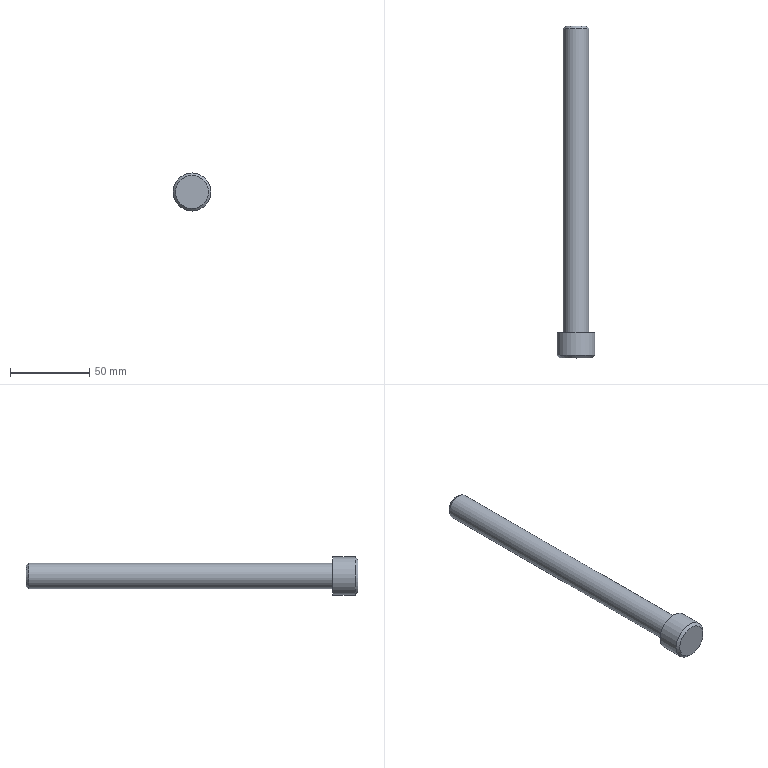Part | STEP file | SCREW-1_id382_x_t | 1 solid | 7 faces | box 24 x 209.351 x 24 mm | volume 45976 mm3 | plane 3 | cone 2 | cylinder 2 | commonest cylinder face diameters 16 x1 24 x1
STEP:
#1=CARTESIAN_POINT('',(165.,-290.,10.4));
#2=VERTEX_POINT('',#1);
#3=CARTESIAN_POINT('',(165.,-290.,0.));
#4=DIRECTION('',(0.,1.,0.));
#5=DIRECTION('',(0.,0.,1.));
#6=AXIS2_PLACEMENT_3D('',#3,#4,#5);
#7=CIRCLE('',#6,10.4);
#8=EDGE_CURVE('',#2,#2,#7,.T.);
#9=ORIENTED_EDGE('',*,*,#8,.F.);
#10=EDGE_LOOP('',(#9));
#11=FACE_OUTER_BOUND('',#10,.T.);
#12=CARTESIAN_POINT('',(165.,-290.,0.));
#13=DIRECTION('',(0.,1.,0.));
#14=DIRECTION('',(0.,0.,1.));
#15=AXIS2_PLACEMENT_3D('',#12,#13,#14);
#16=PLANE('',#15);
#17=ADVANCED_FACE('',(#11),#16,.F.);
#18=CARTESIAN_POINT('',(165.,-288.4,12.));
#19=VERTEX_POINT('',#18);
#20=CARTESIAN_POINT('',(165.,-288.4,0.));
#21=DIRECTION('',(0.,1.,0.));
#22=DIRECTION('',(0.,0.,1.));
#23=AXIS2_PLACEMENT_3D('',#20,#21,#22);
#24=CIRCLE('',#23,12.);
#25=EDGE_CURVE('',#19,#19,#24,.T.);
#26=ORIENTED_EDGE('',*,*,#25,.F.);
#27=EDGE_LOOP('',(#26));
#28=FACE_BOUND('',#27,.T.);
#29=ORIENTED_EDGE('',*,*,#8,.T.);
#30=EDGE_LOOP('',(#29));
#31=FACE_BOUND('',#30,.T.);
#32=CARTESIAN_POINT('',(165.,-288.4,0.));
#33=DIRECTION('',(0.,1.,0.));
#34=DIRECTION('',(0.,0.,1.));
#35=AXIS2_PLACEMENT_3D('',#32,#33,#34);
#36=CONICAL_SURFACE('',#35,12.,45.);
#37=ADVANCED_FACE('',(#28,#31),#36,.T.);
#38=CARTESIAN_POINT('',(165.,-274.,12.));
#39=VERTEX_POINT('',#38);
#40=CARTESIAN_POINT('',(165.,-274.,0.));
#41=DIRECTION('',(0.,1.,0.));
#42=DIRECTION('',(0.,0.,1.));
#43=AXIS2_PLACEMENT_3D('',#40,#41,#42);
#44=CIRCLE('',#43,12.);
#45=EDGE_CURVE('',#39,#39,#44,.T.);
#46=ORIENTED_EDGE('',*,*,#45,.F.);
#47=EDGE_LOOP('',(#46));
#48=FACE_BOUND('',#47,.T.);
#49=ORIENTED_EDGE('',*,*,#25,.T.);
#50=EDGE_LOOP('',(#49));
#51=FACE_BOUND('',#50,.T.);
#52=CARTESIAN_POINT('',(165.,-70.182,0.));
#53=DIRECTION('',(0.,1.,0.));
#54=DIRECTION('',(0.,0.,1.));
#55=AXIS2_PLACEMENT_3D('',#52,#53,#54);
#56=CYLINDRICAL_SURFACE('',#55,12.);
#57=ADVANCED_FACE('',(#48,#51),#56,.T.);
#58=CARTESIAN_POINT('',(165.,-80.649,-6.8));
#59=VERTEX_POINT('',#58);
#60=CARTESIAN_POINT('',(165.,-80.649,0.));
#61=DIRECTION('',(0.,-1.,0.));
#62=DIRECTION('',(0.,0.,-1.));
#63=AXIS2_PLACEMENT_3D('',#60,#61,#62);
#64=CIRCLE('',#63,6.8);
#65=EDGE_CURVE('',#59,#59,#64,.T.);
#66=ORIENTED_EDGE('',*,*,#65,.F.);
#67=EDGE_LOOP('',(#66));
#68=FACE_OUTER_BOUND('',#67,.T.);
#69=CARTESIAN_POINT('',(165.,-80.649,0.));
#70=DIRECTION('',(0.,1.,0.));
#71=DIRECTION('',(0.,0.,1.));
#72=AXIS2_PLACEMENT_3D('',#69,#70,#71);
#73=PLANE('',#72);
#74=ADVANCED_FACE('',(#68),#73,.T.);
#75=CARTESIAN_POINT('',(165.,-274.,8.));
#76=VERTEX_POINT('',#75);
#77=CARTESIAN_POINT('',(165.,-274.,0.));
#78=DIRECTION('',(0.,1.,0.));
#79=DIRECTION('',(0.,0.,1.));
#80=AXIS2_PLACEMENT_3D('',#77,#78,#79);
#81=CIRCLE('',#80,8.);
#82=EDGE_CURVE('',#76,#76,#81,.T.);
#83=ORIENTED_EDGE('',*,*,#82,.F.);
#84=EDGE_LOOP('',(#83));
#85=FACE_BOUND('',#84,.T.);
#86=ORIENTED_EDGE('',*,*,#45,.T.);
#87=EDGE_LOOP('',(#86));
#88=FACE_BOUND('',#87,.T.);
#89=CARTESIAN_POINT('',(165.,-274.,0.));
#90=DIRECTION('',(0.,1.,0.));
#91=DIRECTION('',(0.,0.,1.));
#92=AXIS2_PLACEMENT_3D('',#89,#90,#91);
#93=PLANE('',#92);
#94=ADVANCED_FACE('',(#85,#88),#93,.T.);
#95=ORIENTED_EDGE('',*,*,#65,.T.);
#96=EDGE_LOOP('',(#95));
#97=FACE_BOUND('',#96,.T.);
#98=CARTESIAN_POINT('',(165.,-82.249,8.));
#99=VERTEX_POINT('',#98);
#100=CARTESIAN_POINT('',(165.,-82.249,0.));
#101=DIRECTION('',(0.,-1.,0.));
#102=DIRECTION('',(0.,0.,1.));
#103=AXIS2_PLACEMENT_3D('',#100,#101,#102);
#104=CIRCLE('',#103,8.);
#105=EDGE_CURVE('',#99,#99,#104,.T.);
#106=ORIENTED_EDGE('',*,*,#105,.F.);
#107=EDGE_LOOP('',(#106));
#108=FACE_BOUND('',#107,.T.);
#109=CARTESIAN_POINT('',(165.,-82.249,0.));
#110=DIRECTION('',(0.,-1.,0.));
#111=DIRECTION('',(0.,0.,-1.));
#112=AXIS2_PLACEMENT_3D('',#109,#110,#111);
#113=CONICAL_SURFACE('',#112,8.,36.87);
#114=ADVANCED_FACE('',(#97,#108),#113,.T.);
#115=ORIENTED_EDGE('',*,*,#105,.T.);
#116=EDGE_LOOP('',(#115));
#117=FACE_BOUND('',#116,.T.);
#118=ORIENTED_EDGE('',*,*,#82,.T.);
#119=EDGE_LOOP('',(#118));
#120=FACE_BOUND('',#119,.T.);
#121=CARTESIAN_POINT('',(165.,-70.182,0.));
#122=DIRECTION('',(0.,1.,0.));
#123=DIRECTION('',(0.,0.,1.));
#124=AXIS2_PLACEMENT_3D('',#121,#122,#123);
#125=CYLINDRICAL_SURFACE('',#124,8.);
#126=ADVANCED_FACE('',(#117,#120),#125,.T.);
#127=CLOSED_SHELL('',(#17,#37,#57,#74,#94,#114,#126));
#128=MANIFOLD_SOLID_BREP('',#127);
#129=(LENGTH_UNIT()NAMED_UNIT(*)SI_UNIT(.MILLI.,.METRE.));
#130=UNCERTAINTY_MEASURE_WITH_UNIT(LENGTH_MEASURE(0.00002),#129,'','');
#131=(NAMED_UNIT(*)PLANE_ANGLE_UNIT()SI_UNIT($,.RADIAN.));
#132=PLANE_ANGLE_MEASURE_WITH_UNIT(PLANE_ANGLE_MEASURE(0.01745),#131);
#133=DIMENSIONAL_EXPONENTS(0.,0.,0.,0.,0.,0.,0.);
#134=(CONVERSION_BASED_UNIT('DEGREE',#132)NAMED_UNIT(#133)PLANE_ANGLE_UNIT());
#135=(NAMED_UNIT(*)SI_UNIT($,.STERADIAN.)SOLID_ANGLE_UNIT());
#136=(GEOMETRIC_REPRESENTATION_CONTEXT(3)GLOBAL_UNCERTAINTY_ASSIGNED_CONTEXT((#130))GLOBAL_UNIT_ASSIGNED_CONTEXT((#129,#134,#135))REPRESENTATION_CONTEXT('',''));
#137=ADVANCED_BREP_SHAPE_REPRESENTATION('',(#128),#136);